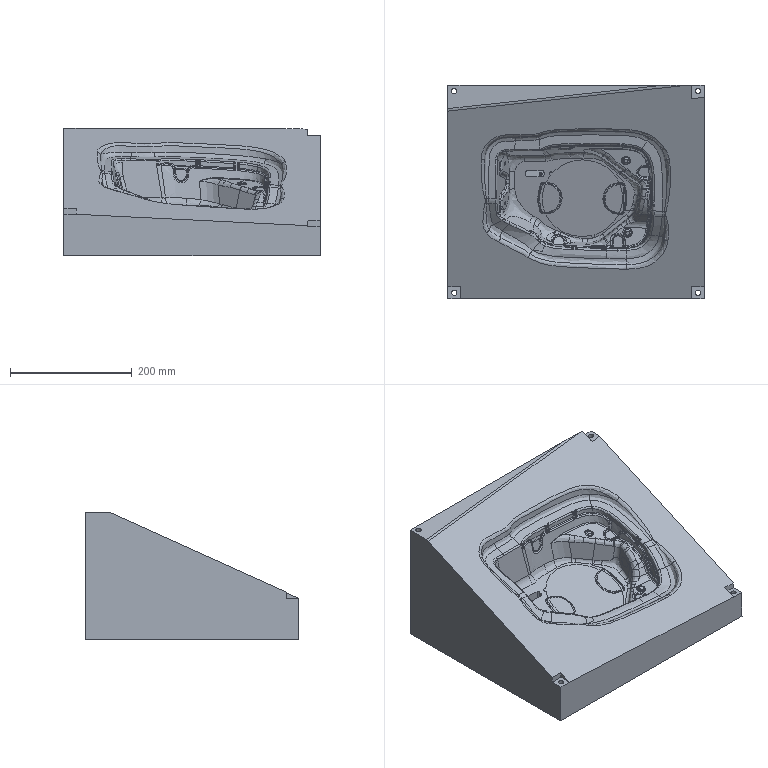NC program | NX | posted with a generic post | part box 420 x 350 x 208.3 mm
Lines 1 to 936 of 93858:
N10 G17 G21 G94 G90
(CAVITY_MILL , TOOL : D40R5)
N12 T00 M6
N14 G54
N16 G17 G0 G90 X29.768 Y-202.884 S1400 M3
N18 G43 Z220. H0
N20 Z207.579
N22 G94 G1 Z207.379 F2600.
N24 Y-18.884
N26 X51.191
N28 G3 X53.878 Y-16.197 R2.7
N30 G1 Y-15.745
N32 G3 X50.9 Y-13.072 R2.7
N34 G1 X8.281 Y-17.689
N36 G3 X8.346 Y-18.884 R0.6
N38 G1 X18.776
N40 G2 X20.896 Y-19.763 R3.
N42 G1 X38.64 Y-37.506
N44 G3 X40.76 Y-38.384 R3.
N46 G1 X70.391
N48 G3 X73.378 Y-35.397 R3.
N50 G1 Y5.647
N52 G3 X70.068 Y8.619 R3.
N54 G1 X-70.714 Y-6.632
N56 G3 X-73.378 Y-9.6 R3.
N58 G1 Y-23.724
N60 X-73.388 Y-23.824
N62 X-73.311 Y-23.887
N64 X-73.154 Y-24.042
N66 G2 X-73.047 Y-24.285 R0.365
N68 G3 X-64.931 Y-31.456 R7.5
N70 G1 X0.572 Y-26.002
N72 G3 X7.424 Y-17.906 R7.5
N74 X-0.673 Y-11.054 R7.5
N76 G1 X-66.176 Y-16.508
N78 G3 X-73.049 Y-23.729 R7.5
N80 G1 X-73.041 Y-23.825
N82 X-73.117 Y-23.884
N84 X-73.27 Y-24.036
N86 G3 X-73.378 Y-24.297 R0.369
N88 G1 Y-35.397
N90 G3 X-70.391 Y-38.384 R3.
N92 G1 X18.777
N94 G2 X20.896 Y-39.262 R3.
N96 G1 X38.64 Y-57.006
N98 G3 X40.76 Y-57.884 R3.
N100 G1 X89.891
N102 G3 X92.878 Y-54.897 R3.
N104 G1 Y27.373
N106 G3 X89.567 Y30.345 R3.
N108 G1 X-90.214 Y10.87
N110 G3 X-92.878 Y7.901 R3.
N112 G1 Y-54.897
N114 G3 X-89.891 Y-57.884 R3.
N116 G1 X18.777
N118 G2 X20.896 Y-58.762 R3.
N120 G1 X38.64 Y-76.507
N122 G3 X40.76 Y-77.384 R3.
N124 G1 X109.39
N126 G3 X112.378 Y-74.396 R3.
N128 G1 Y49.099
N130 G3 X109.067 Y52.071 R3.
N132 G1 X-109.713 Y28.372
N134 G3 X-112.378 Y25.402 R3.
N136 G1 Y-74.396
N138 G3 X-109.39 Y-77.384 R3.
N140 G1 X18.777
N142 G2 X20.896 Y-78.262 R3.
N144 G1 X38.641 Y-96.007
N146 G3 X40.76 Y-96.884 R3.
N148 G1 X128.889
N150 G3 X131.878 Y-93.895 R3.
N152 G1 Y70.825
N154 G3 X128.566 Y73.798 R3.
N156 G1 X-129.212 Y45.873
N158 G3 X-131.878 Y42.903 R3.
N160 G1 Y-93.895
N162 G3 X-128.889 Y-96.884 R3.
N164 G1 X18.777
N166 G2 X20.896 Y-97.762 R3.
N168 G1 X38.641 Y-115.507
N170 G3 X40.759 Y-116.384 R3.
N172 G1 X148.389
N174 G3 X151.378 Y-113.394 R3.
N176 G1 Y92.551
N178 G3 X148.065 Y95.524 R3.
N180 G1 X-148.712 Y63.375
N182 G3 X-151.378 Y60.404 R3.
N184 G1 Y-113.394
N186 G3 X-148.389 Y-116.384 R3.
N188 G1 X18.777
N190 G2 X20.896 Y-117.262 R3.
N192 G1 X38.641 Y-135.007
N194 G3 X40.759 Y-135.884 R3.
N196 G1 X167.887
N198 G3 X170.878 Y-132.893 R3.
N200 G1 Y114.276
N202 G3 X167.564 Y117.251 R3.
N204 G1 X-168.21 Y80.877
N206 G3 X-170.878 Y77.905 R3.
N208 G1 Y-132.893
N210 G3 X-167.887 Y-135.884 R3.
N212 G1 X18.777
N214 G2 X20.896 Y-136.762 R3.
N216 G1 X38.641 Y-154.507
N218 G3 X40.759 Y-155.384 R3.
N220 G1 X187.386
N222 G3 X190.378 Y-152.392 R3.
N224 G1 Y136.034
N226 G3 X186.964 Y138.997 R3.
N228 G2 X185.116 Y138.766 R56.173
N230 G1 X-187.709 Y98.379
N232 G3 X-190.378 Y95.405 R3.
N234 G1 Y-152.392
N236 G3 X-187.386 Y-155.384 R3.
N238 G1 X18.777
N240 G2 X20.896 Y-156.262 R3.
N242 G1 X38.641 Y-174.007
N244 G3 X40.759 Y-174.884 R3.
N246 G1 X209.878
N248 Y174.884
N250 X206.453
N252 G3 X194.644 Y192.884 R19.421
N254 G1 X168.914
N256 G2 X180.303 Y192.147 R416.473
N258 X192.1 Y189.688 R47.532
N260 X192.878 Y160.64 R15.521
N262 X183.016 Y158.153 R36.673
N264 G1 X140.642 Y153.562
N266 X-208.152 Y115.779
N268 G2 X-224.948 Y124.071 R17.869
N270 X-227.878 Y131.354 R23.652
N272 G1 Y121.423
N274 G3 X-209.878 Y111.801 R21.769
N276 G1 Y-174.884
N278 X49.768
N280 Y-202.884
N282 Z207.579
N284 G0 Z208.6
N286 X35.422 Y-203.869
N288 Z206.657
N290 G1 Z206.457
N292 X35.421 Y-19.869
N294 X52.48
N296 G3 X54.868 Y-17.481 R2.4
N298 G1 Y-17.374
N300 G3 X52.221 Y-14.998 R2.4
N302 G1 X18.297 Y-18.673
N304 G3 X18.361 Y-19.869 R0.6
N306 G1 X24.429
N308 G2 X26.549 Y-20.747 R3.
N310 G1 X44.293 Y-38.491
N312 G3 X46.412 Y-39.369 R3.
N314 G1 X71.381
N316 G3 X74.368 Y-36.382 R3.
N318 G1 Y3.685
N320 G3 X71.058 Y6.656 R3.
N322 G1 X-71.704 Y-8.809
N324 G3 X-74.368 Y-11.777 R3.
N326 G1 Y-24.61
N328 X-74.379 Y-24.708
N330 X-74.302 Y-24.769
N332 X-74.15 Y-24.921
N334 G2 X-74.045 Y-25.158 R0.356
N336 G3 X-66.039 Y-32.344 R7.5
N338 G1 X10.486 Y-27.101
N340 G3 X17.455 Y-19.106 R7.5
N342 X9.46 Y-12.136 R7.5
N344 G1 X-67.064 Y-17.379
N346 G3 X-74.047 Y-24.615 R7.5
N348 G1 X-74.038 Y-24.709
N350 X-74.113 Y-24.767
N352 X-74.262 Y-24.915
N354 G3 X-74.368 Y-25.169 R0.359
N356 G1 Y-36.382
N358 G3 X-71.381 Y-39.37 R3.
N360 G1 X24.429 Y-39.369
N362 G2 X26.548 Y-40.247 R3.
N364 G1 X44.293 Y-57.991
N366 G3 X46.412 Y-58.869 R3.
N368 G1 X90.88
N370 G3 X93.868 Y-55.881 R3.
N372 G1 Y25.411
N374 G3 X90.557 Y28.383 R3.
N376 G1 X-91.203 Y8.693
N378 G3 X-93.868 Y5.724 R3.
N380 G1 Y-55.882
N382 G3 X-90.88 Y-58.87 R3.
N384 G1 X24.429 Y-58.869
N386 G2 X26.548 Y-59.747 R3.
N388 G1 X44.293 Y-77.491
N390 G3 X46.412 Y-78.369 R3.
N392 G1 X110.38
N394 G3 X113.368 Y-75.38 R3.
N396 G1 Y47.137
N398 G3 X110.057 Y50.109 R3.
N400 G1 X-110.703 Y26.195
N402 G3 X-113.368 Y23.225 R3.
N404 G1 Y-75.382
N406 G3 X-110.38 Y-78.37 R3.
N408 G1 X24.43 Y-78.369
N410 G2 X26.548 Y-79.247 R3.
N412 G1 X44.293 Y-96.991
N414 G3 X46.412 Y-97.869 R3.
N416 G1 X129.879
N418 G3 X132.868 Y-94.88 R3.
N420 G1 Y68.863
N422 G3 X129.556 Y71.835 R3.
N424 G1 X-130.202 Y43.697
N426 G3 X-132.868 Y40.726 R3.
N428 G1 Y-94.881
N430 G3 X-129.879 Y-97.87 R3.
N432 G1 X24.43 Y-97.869
N434 G2 X26.549 Y-98.747 R3.
N436 G1 X44.293 Y-116.491
N438 G3 X46.412 Y-117.369 R3.
N440 G1 X149.378 Y-117.368
N442 G3 X152.368 Y-114.379 R3.
N444 G1 Y90.588
N446 G3 X149.055 Y93.562 R3.
N448 G1 X-149.701 Y61.198
N450 G3 X-152.368 Y58.227 R3.
N452 G1 Y-114.38
N454 G3 X-149.378 Y-117.37 R3.
N456 G1 X24.43 Y-117.369
N458 G2 X26.548 Y-118.247 R3.
N460 G1 X44.293 Y-135.991
N462 G3 X46.412 Y-136.869 R3.
N464 G1 X168.877 Y-136.868
N466 G3 X171.868 Y-133.877 R3.
N468 G1 Y112.314
N470 G3 X168.554 Y115.288 R3.
N472 G1 X-169.2 Y78.7
N474 G3 X-171.868 Y75.728 R3.
N476 G1 Y-133.879
N478 G3 X-168.877 Y-136.87 R3.
N480 G1 X24.43 Y-136.869
N482 G2 X26.549 Y-137.747 R3.
N484 G1 X44.294 Y-155.491
N486 G3 X46.412 Y-156.369 R3.
N488 G1 X188.376 Y-156.368
N490 G3 X191.368 Y-153.376 R3.
N492 G1 Y134.039
N494 G3 X188.053 Y137.014 R3.
N496 G1 X-188.699 Y96.202
N498 G3 X-191.368 Y93.228 R3.
N500 G1 Y-153.378
N502 G3 X-188.376 Y-156.37 R3.
N504 G1 X24.43 Y-156.369
N506 G2 X26.549 Y-157.247 R3.
N508 G1 X44.294 Y-174.992
N510 G3 X46.412 Y-175.869 R3.
N512 G1 X210.006 Y-175.868
N514 G3 X210.868 Y-175.006 R0.862
N516 G1 Y168.559
N518 G3 X200.957 Y193.868 R21.836
N520 G1 X173.976
N522 G2 X176.105 Y193.795 R853.255
N524 X191.621 Y192.844 R322.887
N526 X201.587 Y161.292 R17.936
N528 X191.869 Y157.042 R17.903
N530 G1 X-208.131 Y113.711
N532 G2 X-224.204 Y120.659 R18.312
N534 G1 X-224.439 Y120.969
N536 G2 X-228.671 Y130.274 R22.991
N538 X-228.868 Y131.299 R30.896
N540 G1 Y120.513
N542 G3 X-227.544 Y118.61 R26.891
N544 G1 X-227.275 Y118.255
N546 G3 X-210.868 Y109.762 R22.212
N548 G1 Y-175.006
N550 G3 X-210.007 Y-175.868 R0.862
N552 G1 X-208.096 Y-175.87
N554 X55.421 Y-175.869
N556 X55.422 Y-203.869
N558 Z206.657
N560 G0 Z207.679
N562 X31.077 Y-204.468
N564 Z205.736
N566 G1 Z205.536
N568 Y-176.468
N570 X31.605 Y-19.272
N572 G3 X31.67 Y-20.468 R0.6
N574 G1 X53.974
N576 G3 X55.465 Y-18.977 R1.5
N578 G1 Y-18.35
N580 G3 X53.812 Y-16.867 R1.5
N582 G1 X42.511 Y-18.091
N584 G2 X40.345 Y-17.474 R3.
N586 G1 X20.176 Y-1.747
N588 G3 X18.01 Y-1.131 R3.
N590 G1 X-72.3 Y-10.914
N592 G3 X-74.965 Y-13.882 R3.
N594 G1 Y-25.123
N596 X-74.975 Y-25.219
N598 X-74.9 Y-25.28
N600 X-74.75 Y-25.428
N602 G2 X-74.648 Y-25.662 R0.35
N604 G3 X-66.734 Y-32.859 R7.5
N606 G1 X23.706 Y-27.795
N608 G3 X30.775 Y-19.888 R7.5
N610 X22.868 Y-12.818 R7.5
N612 G1 X-67.573 Y-17.882
N614 G3 X-74.649 Y-25.128 R7.5
N616 G1 X-74.64 Y-25.221
N618 X-74.714 Y-25.277
N620 X-74.861 Y-25.423
N622 G3 X-74.965 Y-25.672 R0.353
N624 G1 Y-36.981
N626 G3 X-71.977 Y-39.968 R3.
N628 G1 X71.977
N630 G3 X74.965 Y-36.981 R3.
N632 G1 Y1.709
N634 G3 X71.654 Y4.68 R3.
N636 G1 X39.843 Y1.234
N638 G2 X37.641 Y1.879 R3.
N640 G1 X18.089 Y17.609
N642 G3 X15.888 Y18.253 R3.
N644 G1 X-91.8 Y6.588
N646 G3 X-94.465 Y3.619 R3.
N648 G1 Y-56.48
N650 G3 X-91.477 Y-59.468 R3.
N652 G1 X91.477
N654 G3 X94.465 Y-56.48 R3.
N656 G1 Y23.435
N658 G3 X91.154 Y26.407 R3.
N660 G1 X37.743 Y20.621
N662 G2 X35.541 Y21.265 R3.
N664 G1 X15.989 Y36.996
N666 G3 X13.788 Y37.64 R3.
N668 G1 X-111.299 Y24.09
N670 G3 X-113.965 Y21.12 R3.
N672 G1 Y-75.98
N674 G3 X-110.976 Y-78.968 R3.
N676 G1 X110.976
N678 G3 X113.965 Y-75.98 R3.
N680 G1 Y45.161
N682 G3 X110.653 Y48.133 R3.
N684 G1 X35.643 Y40.007
N686 G2 X33.441 Y40.652 R3.
N688 G1 X13.889 Y56.382
N690 G3 X11.688 Y57.027 R3.
N692 G1 X-130.799 Y41.591
N694 G3 X-133.465 Y38.621 R3.
N696 G1 Y-95.479
N698 G3 X-130.476 Y-98.468 R3.
N700 G1 X130.476
N702 G3 X133.465 Y-95.479 R3.
N704 G1 Y66.887
N706 G3 X130.152 Y69.859 R3.
N708 G1 X33.543 Y59.394
N710 G2 X31.341 Y60.038 R3.
N712 G1 X11.789 Y75.769
N714 G3 X9.588 Y76.413 R3.
N716 G1 X-150.298 Y59.093
N718 G3 X-152.965 Y56.122 R3.
N720 G1 Y-114.978
N722 G3 X-149.975 Y-117.968 R3.
N724 G1 X149.975
N726 G3 X152.965 Y-114.978 R3.
N728 G1 Y88.612
N730 G3 X149.652 Y91.586 R3.
N732 G1 X31.442 Y78.781
N734 G2 X29.241 Y79.425 R3.
N736 G1 X9.689 Y95.156
N738 G3 X7.488 Y95.8 R3.
N740 G1 X-169.797 Y76.595
N742 G3 X-172.465 Y73.623 R3.
N744 G1 Y-134.477
N746 G3 X-169.474 Y-137.468 R3.
N748 G1 X169.474
N750 G3 X172.465 Y-134.477 R3.
N752 G1 Y110.338
N754 G3 X169.151 Y113.312 R3.
N756 G1 X29.342 Y98.167
N758 G2 X27.141 Y98.812 R3.
N760 G1 X7.588 Y114.542
N762 G3 X5.388 Y115.186 R3.
N764 G1 X-189.295 Y94.097
N766 G3 X-191.965 Y91.123 R3.
N768 G1 Y-153.976
N770 G3 X-188.972 Y-156.968 R3.
N772 G1 X188.972
N774 G3 X191.965 Y-153.976 R3.
N776 G1 Y132.063
N778 G3 X188.649 Y135.039 R3.
N780 G1 X27.242 Y117.554
N782 G2 X25.041 Y118.198 R3.
N784 G1 X5.488 Y133.929
N786 G3 X3.288 Y134.573 R3.
N788 G1 X-208.131 Y111.671
N790 G2 X-224.204 Y118.619 R18.312
N792 G1 X-224.379 Y118.849
N794 G2 X-229.465 Y130.885 R26.559
N796 G1 Y119.448
N798 G3 X-227.487 Y116.494 R30.459
N800 G1 X-227.275 Y116.215
N802 G3 X-211.465 Y107.759 R22.212
N804 G1 Y-175.091
N806 G3 X-211.039 Y-176.036 R1.546
N808 X-210.563 Y-176.352 R2.162
N810 X-209.938 Y-176.468 R1.743
N812 G1 X210.065
N814 G3 X211.465 Y-175.101 R1.489
N816 G1 Y166.887
N818 G3 X202.132 Y194.468 R22.95
N820 G1 X179.222
N822 G2 X190.898 Y194.019 R642.084
N824 X207.353 Y167.146 R19.05
N826 G1 X207.136 Y166.668
N828 G2 X201. Y158.77 R21.899
N830 X191.954 Y155.011 R17.364
N832 G1 X152.85 Y150.775
N834 X-5.669 Y133.603
N836 X-3.515 Y113.719
N838 Z205.736
N840 G0 Z206.757
N842 X46.69 Y-204.817
N844 Z204.814
N846 G1 Z204.614
N848 Y-176.817
N850 X47.284 Y-20.817
N852 X54.922
N854 G3 X55.815 Y-19.924 R0.9
N856 G1 Y-19.686
N858 G3 X54.825 Y-18.797 R0.9
N860 G1 X47.219 Y-19.621
N862 G3 X46.69 Y-20.249 R0.6
N864 G1 X55.625 Y-38.629
N866 G3 X58.322 Y-40.317 R3.
N868 G1 X72.328
N870 G3 X75.315 Y-37.33 R3.
N872 G1 Y-0.293
N874 G3 X72.004 Y2.678 R3.
N876 G1 X-72.651 Y-12.992
N878 G3 X-75.315 Y-15.961 R3.
N880 G1 Y-37.33
N882 G3 X-72.328 Y-40.317 R3.
N884 G1 X-58.758
N886 G3 X-56.608 Y-39.409 R3.
N888 G1 X-51.191 Y-33.843
N890 G2 X-49.203 Y-32.939 R3.
N892 G1 X39.306 Y-28.159
N894 G3 X46.391 Y-20.266 R7.5
N896 X38.497 Y-13.181 R7.5
N898 G1 X-54.739 Y-18.216
N900 G3 X-57.836 Y-32.338 R7.5
N902 G2 X-57.012 Y-32.977 R3.
N904 G1 X-51.262 Y-39.33
N906 G3 X-49.037 Y-40.317 R3.
N908 G1 X35.699
N910 G2 X37.818 Y-41.195 R3.
N912 G1 X55.562 Y-58.939
N914 G3 X57.682 Y-59.817 R3.
N916 G1 X91.827
N918 G3 X94.815 Y-56.829 R3.
N920 G1 Y21.433
N922 G3 X91.504 Y24.404 R3.
N924 G1 X-92.15 Y4.509
N926 G3 X-94.815 Y1.541 R3.
N928 G1 Y-56.829
N930 G3 X-91.827 Y-59.817 R3.
N932 G1 X35.699
N934 G2 X37.818 Y-60.695 R3.
N936 G1 X55.563 Y-78.439
N938 G3 X57.682 Y-79.317 R3.
N940 G1 X111.327
N942 G3 X114.315 Y-76.329 R3.
N944 G1 Y43.159
N946 G3 X111.003 Y46.131 R3.
N948 G1 X-111.65 Y22.011
N950 G3 X-114.315 Y19.042 R3.
N952 G1 Y-76.329
N954 G3 X-111.327 Y-79.317 R3.
N956 G1 X35.699
N958 G2 X37.818 Y-80.195 R3.
N960 G1 X55.563 Y-97.939
N962 G3 X57.682 Y-98.817 R3.
N964 G1 X130.826
N966 G3 X133.815 Y-95.828 R3.
N968 G1 Y64.884
N970 G3 X130.503 Y67.857 R3.
N972 G1 X-131.149 Y39.513
N974 G3 X-133.815 Y36.543 R3.
N976 G1 Y-95.828
N978 G3 X-130.826 Y-98.817 R3.
N980 G1 X35.7
N982 G2 X37.818 Y-99.695 R3.
N984 G1 X55.563 Y-117.439
N986 G3 X57.682 Y-118.317 R3.
N988 G1 X150.325
N990 G3 X153.315 Y-115.327 R3.
N992 G1 Y86.61
N994 G3 X150.002 Y89.583 R3.
N996 G1 X-150.648 Y57.015
N998 G3 X-153.315 Y54.043 R3.
N1000 G1 Y-115.327
N1002 G3 X-150.325 Y-118.317 R3.
N1004 G1 X35.7
N1006 G2 X37.818 Y-119.194 R3.
N1008 G1 X55.563 Y-136.939
N1010 G3 X57.682 Y-137.817 R3.
N1012 G1 X169.824
N1014 G3 X172.815 Y-134.826 R3.
N1016 G1 Y108.335
N1018 G3 X169.501 Y111.31 R3.
N1020 G1 X-170.147 Y74.517
N1022 G3 X-172.815 Y71.544 R3.
N1024 G1 Y-134.826
N1026 G3 X-169.824 Y-137.817 R3.
N1028 G1 X35.7
N1030 G2 X37.818 Y-138.694 R3.
N1032 G1 X55.563 Y-156.439
N1034 G3 X57.681 Y-157.317 R3.
N1036 G1 X189.323
N1038 G3 X192.315 Y-154.325 R3.
N1040 G1 Y130.06
N1042 G3 X189. Y133.036 R3.
N1044 G1 X-189.646 Y92.018
N1046 G3 X-192.315 Y89.045 R3.
N1048 G1 Y-154.325
N1050 G3 X-189.323 Y-157.317 R3.
N1052 G1 X35.7
N1054 G2 X37.818 Y-158.194 R3.
N1056 G1 X55.563 Y-175.94
N1058 G3 X57.682 Y-176.817 R3.
N1060 G1 X210.002
N1062 G3 X211.815 Y-175.004 R1.813
N1064 G1 Y165.717
N1066 G3 X212.57 Y168.036 R31.071
N1068 G1 X212.804 Y168.909
N1070 G3 X202.844 Y194.817 R23.588
N1072 G1 X185.702
N1074 X190.497 Y194.701
N1076 G2 X209.037 Y169.919 R19.688
N1078 G1 X208.803 Y169.047
N1080 G2 X204.065 Y159.741 R27.171
N1082 X191.869 Y152.961 R18.343
N1084 G1 X-208.131 Y109.63
N1086 G2 X-224.204 Y116.578 R18.312
N1088 G1 X-225.156 Y117.867
N1090 G2 X-229.201 Y127.173 R28.748
N1092 X-229.815 Y130.388 R38.817
N1094 G1 Y118.031
N1096 G3 X-228.403 Y115.706 R32.648
N1098 G1 X-228.293 Y115.549
N1100 X-227.34 Y114.26
N1102 X-227.275 Y114.174
N1104 G3 X-211.815 Y105.748 R22.212
N1106 G1 Y-175.004
N1108 G3 X-210.002 Y-176.817 R1.813
N1110 G1 X66.69
N1112 Y-204.817
N1114 Z204.814
N1116 G0 Z205.836
N1118 X46.436 Y-204.975
N1120 Z203.893
N1122 G1 Z203.693
N1124 Y-22.475
N1126 X55.981
N1128 G3 X57.472 Y-20.984 R1.5
N1130 G1 Y-20.704
N1132 G3 X55.819 Y-19.221 R1.5
N1134 G1 X36.826 Y-21.279
N1136 G3 X36.765 Y-22.46 R0.6
N1138 G2 X38.226 Y-23.265 R3.
N1140 G1 X54.558 Y-39.596
N1142 G3 X56.678 Y-40.475 R3.
N1144 G1 X72.484
N1146 G3 X75.472 Y-37.487 R3.
N1148 G1 Y-2.317
N1150 G3 X72.161 Y0.654 R3.
N1152 G1 X-72.808 Y-15.05
N1154 G3 X-75.472 Y-18.018 R3.
N1156 G1 Y-37.487
N1158 G3 X-72.484 Y-40.475 R3.
N1160 G1 X-41.376
N1162 G3 X-39.226 Y-39.567 R3.
N1164 G1 X-33.809 Y-34.
N1166 G2 X-31.821 Y-33.097 R3.
N1168 G1 X28.913 Y-29.817
N1170 G3 X35.998 Y-21.923 R7.5
N1172 X28.104 Y-14.838 R7.5
N1174 G1 X-37.357 Y-18.374
N1176 G3 X-40.454 Y-32.495 R7.5
N1178 G2 X-39.63 Y-33.135 R3.
N1180 G1 X-33.88 Y-39.488
N1182 G3 X-31.656 Y-40.475 R3.
N1184 G1 X35.444
N1186 G2 X37.564 Y-41.353 R3.
N1188 G1 X55.308 Y-59.097
N1190 G3 X57.427 Y-59.975 R3.
N1192 G1 X91.984
N1194 G3 X94.972 Y-56.987 R3.
N1196 G1 Y19.409
N1198 G3 X91.661 Y22.381 R3.
N1200 G1 X-92.307 Y2.452
N1202 G3 X-94.972 Y-0.517 R3.
N1204 G1 Y-56.987
N1206 G3 X-91.984 Y-59.975 R3.
N1208 G1 X35.445
N1210 G2 X37.563 Y-60.852 R3.
N1212 G1 X55.308 Y-78.597
N1214 G3 X57.427 Y-79.475 R3.
N1216 G1 X111.483
N1218 G3 X114.472 Y-76.486 R3.
N1220 G1 Y41.135
N1222 G3 X111.16 Y44.107 R3.
N1224 G1 X-111.806 Y19.954
N1226 G3 X-114.472 Y16.984 R3.
N1228 G1 Y-76.486
N1230 G3 X-111.483 Y-79.475 R3.
N1232 G1 X35.445
N1234 G2 X37.563 Y-80.352 R3.
N1236 G1 X55.308 Y-98.097
N1238 G3 X57.427 Y-98.975 R3.
N1240 G1 X130.983
N1242 G3 X133.972 Y-95.986 R3.
N1244 G1 Y62.861
N1246 G3 X130.66 Y65.834 R3.
N1248 G1 X-131.306 Y37.456
N1250 G3 X-133.972 Y34.485 R3.
N1252 G1 Y-95.986
N1254 G3 X-130.983 Y-98.975 R3.
N1256 G1 X35.445
N1258 G2 X37.563 Y-99.852 R3.
N1260 G1 X55.308 Y-117.597
N1262 G3 X57.427 Y-118.475 R3.
N1264 G1 X150.482
N1266 G3 X153.472 Y-115.485 R3.
N1268 G1 Y84.586
N1270 G3 X150.159 Y87.56 R3.
N1272 G1 X-150.805 Y54.957
N1274 G3 X-153.472 Y51.986 R3.
N1276 G1 Y-115.485
N1278 G3 X-150.482 Y-118.475 R3.
N1280 G1 X35.445
N1282 G2 X37.563 Y-119.352 R3.
N1284 G1 X55.308 Y-137.097
N1286 G3 X57.427 Y-137.975 R3.
N1288 G1 X169.981
N1290 G3 X172.972 Y-134.984 R3.
N1292 G1 Y106.312
N1294 G3 X169.658 Y109.286 R3.
N1296 G1 X-170.304 Y72.459
N1298 G3 X-172.972 Y69.487 R3.
N1300 G1 Y-134.984
N1302 G3 X-169.981 Y-137.975 R3.
N1304 G1 X35.445
N1306 G2 X37.563 Y-138.852 R3.
N1308 G1 X55.308 Y-156.597
N1310 G3 X57.427 Y-157.475 R3.
N1312 G1 X189.48
N1314 G3 X192.472 Y-154.482 R3.
N1316 G1 Y128.037
N1318 G3 X189.156 Y131.013 R3.
N1320 G1 X-189.803 Y89.961
N1322 G3 X-192.472 Y86.987 R3.
N1324 G1 Y-154.482
N1326 G3 X-189.48 Y-157.475 R3.
N1328 G1 X35.445
N1330 G2 X37.563 Y-158.352 R3.
N1332 G1 X55.308 Y-176.097
N1334 G3 X57.427 Y-176.975 R3.
N1336 G1 X209.995
N1338 G3 X211.972 Y-174.998 R1.976
N1340 G1 Y164.107
N1342 G3 X213.483 Y169.851 R33.937
N1344 X203.343 Y194.975 R24.046
N1346 G1 X192.431
N1348 G2 X209.654 Y170.597 R20.146
N1350 X205.554 Y159.741 R30.037
N1352 X191.869 Y150.92 R18.75
N1354 G1 X-208.131 Y107.59
N1356 G2 X-222.839 Y113.01 R17.846
N1358 X-227.601 Y120.322 R23.615
N1360 X-229.972 Y129.054 R35.914
N1362 G1 Y116.237
N1364 G3 X-225.658 Y110.315 R27.515
N1366 X-211.972 Y103.693 R21.746
N1368 G1 Y-174.998
N1370 G3 X-209.995 Y-176.975 R1.976
N1372 G1 X66.436
N1374 Y-204.975
N1376 Z203.893
N1378 G0 Z204.914
N1380 X54.929 Y-204.997
N1382 Z202.971
N1384 G1 Z202.771
N1386 Y-176.997
N1388 X55.522 Y-22.497
N1390 X56.899
N1392 G3 X57.493 Y-21.903 R0.6
N1394 G1 Y-21.743
N1396 G3 X56.834 Y-21.152 R0.6
N1398 G1 X55.458 Y-21.301
N1400 G3 X54.929 Y-21.929 R0.6
N1402 G1 X63.114 Y-38.806
N1404 G3 X65.813 Y-40.497 R3.
N1406 G1 X72.506
N1408 G3 X75.493 Y-37.509 R3.
N1410 G1 Y-4.355
N1412 G3 X72.183 Y-1.384 R3.
N1414 G1 X-72.833 Y-17.093
N1416 G3 X-75.497 Y-20.061 R3.
N1418 G1 X-75.498 Y-37.509
N1420 G3 X-72.51 Y-40.497 R3.
N1422 G1 X-22.744
N1424 G3 X-20.594 Y-39.589 R3.
N1426 G1 X-15.178 Y-34.022
N1428 G2 X-13.189 Y-33.119 R3.
N1430 G1 X47.545 Y-29.839
N1432 G3 X54.63 Y-21.945 R7.5
N1434 X46.736 Y-14.861 R7.5
N1436 G1 X-18.725 Y-18.396
N1438 G3 X-21.822 Y-32.517 R7.5
N1440 G2 X-20.999 Y-33.157 R3.
N1442 G1 X-15.248 Y-39.51
N1444 G3 X-13.024 Y-40.497 R3.
N1446 G1 X43.938
N1448 G2 X46.057 Y-41.375 R3.
N1450 G1 X63.801 Y-59.119
N1452 G3 X65.921 Y-59.997 R3.
N1454 G1 X92.005
N1456 G3 X94.993 Y-57.009 R3.
N1458 G1 X94.994 Y17.371
N1460 G3 X91.683 Y20.343 R3.
N1462 G1 X-92.333 Y0.409
N1464 G3 X-94.997 Y-2.56 R3.
N1466 G1 X-94.998 Y-57.009
N1468 G3 X-92.01 Y-59.997 R3.
N1470 G1 X43.938
N1472 G2 X46.057 Y-60.874 R3.
N1474 G1 X63.801 Y-78.619
N1476 G3 X65.921 Y-79.497 R3.
N1478 G1 X111.504
N1480 G3 X114.493 Y-76.508 R3.
N1482 G1 X114.494 Y39.097
N1484 G3 X111.182 Y42.069 R3.
N1486 G1 X-111.832 Y17.911
N1488 G3 X-114.497 Y14.941 R3.
N1490 G1 X-114.498 Y-76.508
N1492 G3 X-111.51 Y-79.497 R3.
N1494 G1 X43.938
N1496 G2 X46.057 Y-80.374 R3.
N1498 G1 X63.801 Y-98.119
N1500 G3 X65.921 Y-98.997 R3.
N1502 G1 X131.004
N1504 G3 X133.993 Y-96.008 R3.
N1506 G1 X133.994 Y60.823
N1508 G3 X130.682 Y63.795 R3.
N1510 G1 X-131.331 Y35.412
N1512 G3 X-133.997 Y32.442 R3.
N1514 G1 X-133.998 Y-96.008
N1516 G3 X-131.009 Y-98.997 R3.
N1518 G1 X43.938
N1520 G2 X46.057 Y-99.874 R3.
N1522 G1 X63.801 Y-117.619
N1524 G3 X65.92 Y-118.497 R3.
N1526 G1 X150.503
N1528 G3 X153.492 Y-115.507 R3.
N1530 G1 X153.494 Y82.548
N1532 G3 X150.181 Y85.522 R3.
N1534 G1 X-150.83 Y52.914
N1536 G3 X-153.497 Y49.943 R3.
N1538 G1 X-153.499 Y-115.507
N1540 G3 X-150.509 Y-118.497 R3.
N1542 G1 X43.938
N1544 G2 X46.057 Y-119.374 R3.
N1546 G1 X63.801 Y-137.119
N1548 G3 X65.92 Y-137.997 R3.
N1550 G1 X170.001
N1552 G3 X172.992 Y-135.006 R3.
N1554 G1 X172.994 Y104.274
N1556 G3 X169.68 Y107.248 R3.
N1558 G1 X-170.329 Y70.416
N1560 G3 X-172.996 Y67.444 R3.
N1562 G1 X-172.999 Y-135.006
N1564 G3 X-170.008 Y-137.997 R3.
N1566 G1 X43.938
N1568 G2 X46.057 Y-138.874 R3.
N1570 G1 X63.802 Y-156.619
N1572 G3 X65.92 Y-157.497 R3.
N1574 G1 X189.5
N1576 G3 X192.492 Y-154.504 R3.
N1578 G1 X192.495 Y125.999
N1580 G3 X189.179 Y128.975 R3.
N1582 G1 X-189.827 Y87.918
N1584 G3 X-192.496 Y84.944 R3.
N1586 G1 X-192.499 Y-154.504
N1588 G3 X-189.507 Y-157.497 R3.
N1590 G1 X43.939
N1592 G2 X46.056 Y-158.374 R3.
N1594 G1 X63.802 Y-176.119
N1596 G3 X65.92 Y-176.997 R3.
N1598 G1 X210.002
N1600 G3 X211.992 Y-175.007 R1.99
N1602 G1 X211.995 Y162.192
N1604 G3 X214.219 Y174.22 R41.12
N1606 X203.709 Y194.997 R24.198
N1608 G1 X193.703
N1610 G2 X210.321 Y174.351 R20.298
N1612 X207.685 Y161.79 R37.22
N1614 X202.697 Y154.156 R23.108
N1616 X191.869 Y148.88 R18.058
N1618 G1 X-208.131 Y105.549
N1620 G2 X-224.747 Y113.215 R18.166
N1622 X-229.049 Y122.52 R28.211
N1624 X-229.996 Y127.303 R42.567
N1626 G1 Y114.295
N1628 G3 X-227.937 Y110.97 R32.111
N1630 X-211.996 Y101.669 R22.066
N1632 G1 X-211.999 Y-174.962
N1634 G3 X-211.936 Y-175.485 R2.198
N1636 X-210.095 Y-176.997 R1.987
N1638 G1 X74.929
N1640 Y-204.997
N1642 Z202.971
N1644 G0 Z203.993
N1646 X74.614
N1648 Z202.05
N1650 G1 Z201.85
N1652 Y-176.997
N1654 X72.539 Y-40.496
N1656 G3 X75.493 Y-37.509 R3.
N1658 G1 Y-6.395
N1660 G3 X72.183 Y-3.424 R3.
N1662 G1 X39.311 Y-6.985
N1664 G3 X37.297 Y-8.087 R3.
N1666 G1 X28.882 Y-18.547
N1668 G2 X26.868 Y-19.649 R3.
N1670 G1 X7.301 Y-21.768
N1672 G3 X7.705 Y-29.247 R3.75
N1674 G1 X60.493
N1676 G3 X64.243 Y-25.497 R3.75
N1678 G1 Y-19.779
N1680 G3 X60.089 Y-16.05 R3.75
N1682 G1 X40.523 Y-18.17
N1684 G2 X38.319 Y-17.525 R3.
N1686 G1 X27.86 Y-9.109
N1688 G3 X25.656 Y-8.464 R3.
N1690 G1 X-72.833 Y-19.133
N1692 G3 X-75.497 Y-22.102 R3.
N1694 G1 X-75.498 Y-37.509
N1696 G3 X-72.51 Y-40.497 R3.
N1698 G1 X61.585 Y-40.496
N1700 G2 X63.588 Y-41.265 R3.
N1702 G1 X83.565 Y-59.228
N1704 G3 X85.569 Y-59.997 R3.
N1706 G1 X92.005
N1708 G3 X94.993 Y-57.009 R3.
N1710 G1 X94.994 Y15.331
N1712 G3 X91.683 Y18.302 R3.
N1714 G1 X-92.333 Y-1.632
N1716 G3 X-94.997 Y-4.601 R3.
N1718 G1 X-94.998 Y-57.009
N1720 G3 X-92.01 Y-59.997 R3.
N1722 G1 X63.623
N1724 G2 X65.742 Y-60.874 R3.
N1726 G1 X83.486 Y-78.619
N1728 G3 X85.606 Y-79.497 R3.
N1730 G1 X111.504
N1732 G3 X114.493 Y-76.508 R3.
N1734 G1 X114.494 Y37.056
N1736 G3 X111.182 Y40.029 R3.
N1738 G1 X-111.832 Y15.87
N1740 G3 X-114.497 Y12.901 R3.
N1742 G1 X-114.498 Y-76.508
N1744 G3 X-111.51 Y-79.497 R3.
N1746 G1 X63.623
N1748 G2 X65.742 Y-80.374 R3.
N1750 G1 X83.486 Y-98.119
N1752 G3 X85.606 Y-98.997 R3.
N1754 G1 X131.004
N1756 G3 X133.993 Y-96.008 R3.
N1758 G1 X133.994 Y58.782
N1760 G3 X130.682 Y61.755 R3.
N1762 G1 X-131.331 Y33.372
N1764 G3 X-133.997 Y30.402 R3.
N1766 G1 X-133.998 Y-96.008
N1768 G3 X-131.009 Y-98.997 R3.
N1770 G1 X63.623
N1772 G2 X65.742 Y-99.874 R3.
N1774 G1 X83.487 Y-117.619
N1776 G3 X85.606 Y-118.497 R3.
N1778 G1 X150.503
N1780 G3 X153.492 Y-115.507 R3.
N1782 G1 X153.494 Y80.508
N1784 G3 X150.181 Y83.481 R3.
N1786 G1 X-150.83 Y50.874
N1788 G3 X-153.497 Y47.903 R3.
N1790 G1 X-153.499 Y-115.507
N1792 G3 X-150.509 Y-118.497 R3.
N1794 G1 X63.624
N1796 G2 X65.742 Y-119.374 R3.
N1798 G1 X83.487 Y-137.119
N1800 G3 X85.606 Y-137.997 R3.
N1802 G1 X170.001
N1804 G3 X172.992 Y-135.006 R3.
N1806 G1 X172.994 Y102.233
N1808 G3 X169.68 Y105.208 R3.
N1810 G1 X-170.328 Y68.376
N1812 G3 X-172.996 Y65.403 R3.
N1814 G1 X-172.999 Y-135.006
N1816 G3 X-170.008 Y-137.997 R3.
N1818 G1 X63.624
N1820 G2 X65.742 Y-138.874 R3.
N1822 G1 X83.487 Y-156.619
N1824 G3 X85.606 Y-157.497 R3.
N1826 G1 X189.5
N1828 G3 X192.492 Y-154.504 R3.
N1830 G1 X192.495 Y123.958
N1832 G3 X189.179 Y126.934 R3.
N1834 G1 X-189.827 Y85.877
N1836 G3 X-192.496 Y82.904 R3.
N1838 G1 X-192.499 Y-154.504
N1840 G3 X-189.507 Y-157.497 R3.
N1842 G1 X63.624
N1844 G2 X65.742 Y-158.374 R3.
N1846 G1 X83.487 Y-176.119
N1848 G3 X85.606 Y-176.997 R3.
N1850 G1 X210.002
N1852 G3 X211.992 Y-175.007 R1.99
N1854 G1 X211.995 Y160.095
N1856 G3 X212.527 Y161.763 R31.053
N1858 X214.3 Y174.583 R45.587
N1860 G1 Y175.
N1862 G3 X203.807 Y194.997 R24.3
N1864 G1 X194.036
N1866 G2 X210.4 Y175. R20.4
N1868 G1 Y174.573
N1870 G2 X208.779 Y162.843 R41.687